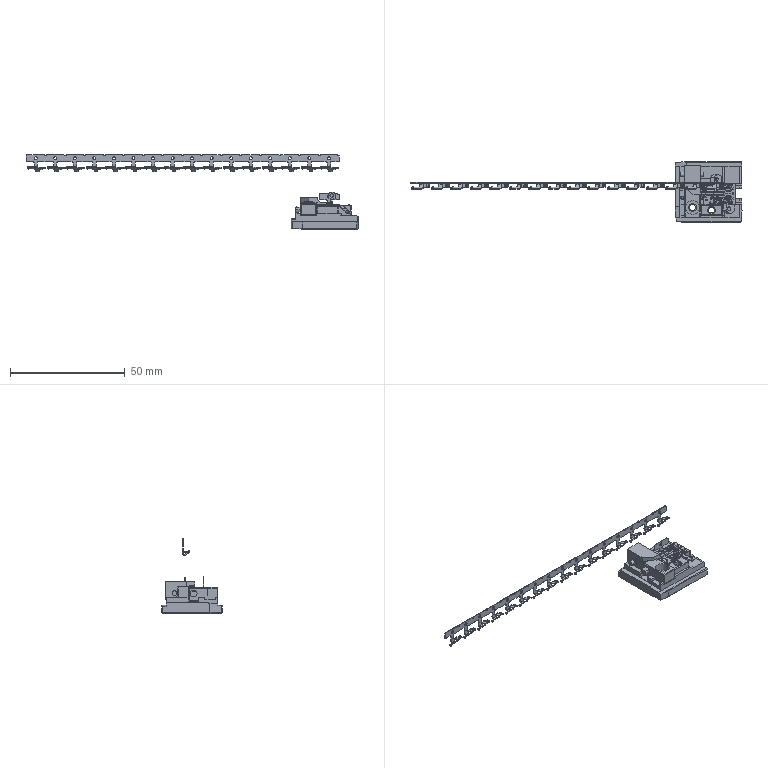Part | NX | 13 solids | 2969 faces | box 144.41 x 26.5 x 32.318 mm | volume 5107 mm3 | plane 1435 | cylinder 1010 | torus 354 | sphere 120 | cone 28 | spline 22 | commonest cylinder face diameters 0.2 x235 0.4 x144 0.5 x113 0.7 x86 1 x67 0.6 x61